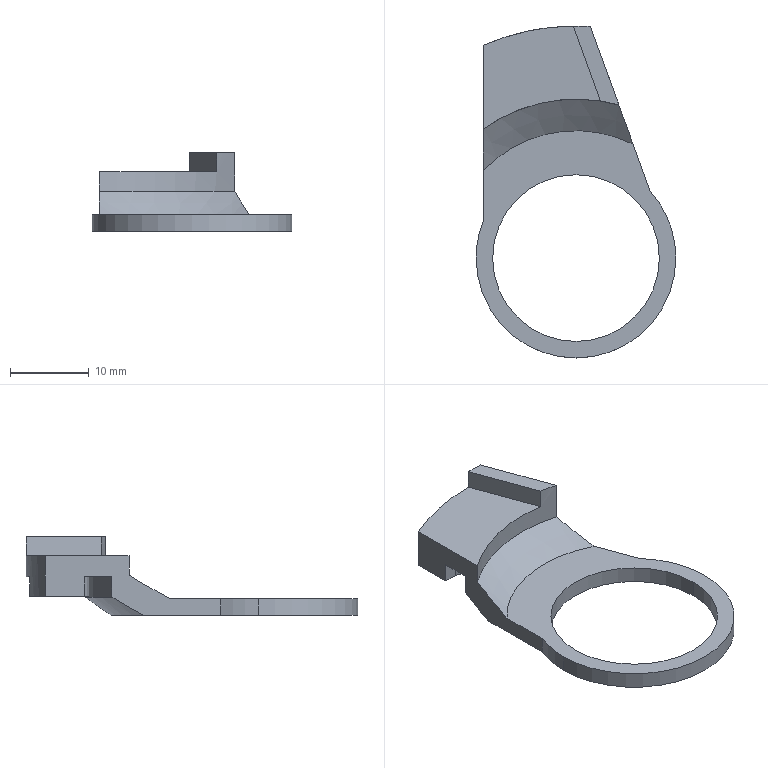Part | STEP file | A22NZ_H_02_LEVER | 1 solid | 23 faces | box 25.4 x 42.2 x 10 mm | volume 1414 mm3 | plane 11 | cylinder 10 | cone 2 | commonest cylinder face diameters 25.4 x3 7.5 x2 21.2 x2 40.4 x1 44 x1 59 x1
STEP:
#1=CARTESIAN_POINT('',(-4.25,25.26,0.3));
#2=VERTEX_POINT('',#1);
#3=CARTESIAN_POINT('',(-10.035,22.11,0.3));
#4=VERTEX_POINT('',#3);
#5=CARTESIAN_POINT('',(-8.,25.26,0.3));
#6=DIRECTION('',(0.,0.,-1.));
#7=DIRECTION('',(-1.,0.,0.));
#8=AXIS2_PLACEMENT_3D('',#5,#6,#7);
#9=CIRCLE('',#8,3.75);
#10=EDGE_CURVE('',#2,#4,#9,.T.);
#11=ORIENTED_EDGE('',*,*,#10,.F.);
#12=CARTESIAN_POINT('',(-4.25,25.26,2.8));
#13=VERTEX_POINT('',#12);
#14=CARTESIAN_POINT('',(-4.25,25.26,0.3));
#15=DIRECTION('',(0.,0.,1.));
#16=VECTOR('',#15,1000.);
#17=LINE('',#14,#16);
#18=EDGE_CURVE('',#2,#13,#17,.T.);
#19=ORIENTED_EDGE('',*,*,#18,.T.);
#20=CARTESIAN_POINT('',(-10.035,22.11,2.8));
#21=VERTEX_POINT('',#20);
#22=CARTESIAN_POINT('',(-8.,25.26,2.8));
#23=DIRECTION('',(0.,0.,-1.));
#24=DIRECTION('',(-1.,0.,0.));
#25=AXIS2_PLACEMENT_3D('',#22,#23,#24);
#26=CIRCLE('',#25,3.75);
#27=EDGE_CURVE('',#13,#21,#26,.T.);
#28=ORIENTED_EDGE('',*,*,#27,.T.);
#29=CARTESIAN_POINT('',(-10.035,22.11,0.3));
#30=DIRECTION('',(0.,0.,1.));
#31=VECTOR('',#30,1000.);
#32=LINE('',#29,#31);
#33=EDGE_CURVE('',#4,#21,#32,.T.);
#34=ORIENTED_EDGE('',*,*,#33,.F.);
#35=EDGE_LOOP('',(#11,#19,#28,#34));
#36=FACE_OUTER_BOUND('',#35,.T.);
#37=CARTESIAN_POINT('',(-8.,25.26,0.3));
#38=DIRECTION('',(0.,0.,1.));
#39=DIRECTION('',(1.,0.,0.));
#40=AXIS2_PLACEMENT_3D('',#37,#38,#39);
#41=CYLINDRICAL_SURFACE('',#40,3.75);
#42=ADVANCED_FACE('',(#36),#41,.T.);
#43=CARTESIAN_POINT('',(10.6,0.,-2.1));
#44=VERTEX_POINT('',#43);
#45=CARTESIAN_POINT('',(-10.6,0.,-2.1));
#46=VERTEX_POINT('',#45);
#47=CARTESIAN_POINT('',(0.,0.,-2.1));
#48=DIRECTION('',(0.,0.,-1.));
#49=DIRECTION('',(-1.,0.,0.));
#50=AXIS2_PLACEMENT_3D('',#47,#48,#49);
#51=CIRCLE('',#50,10.6);
#52=EDGE_CURVE('',#44,#46,#51,.T.);
#53=ORIENTED_EDGE('',*,*,#52,.T.);
#54=CARTESIAN_POINT('',(-10.6,0.,0.));
#55=VERTEX_POINT('',#54);
#56=CARTESIAN_POINT('',(-10.6,0.,-2.1));
#57=DIRECTION('',(0.,0.,1.));
#58=VECTOR('',#57,1000.);
#59=LINE('',#56,#58);
#60=EDGE_CURVE('',#46,#55,#59,.T.);
#61=ORIENTED_EDGE('',*,*,#60,.T.);
#62=CARTESIAN_POINT('',(10.6,0.,0.));
#63=VERTEX_POINT('',#62);
#64=CARTESIAN_POINT('',(0.,0.,0.));
#65=DIRECTION('',(0.,0.,-1.));
#66=DIRECTION('',(-1.,0.,0.));
#67=AXIS2_PLACEMENT_3D('',#64,#65,#66);
#68=CIRCLE('',#67,10.6);
#69=EDGE_CURVE('',#63,#55,#68,.T.);
#70=ORIENTED_EDGE('',*,*,#69,.F.);
#71=CARTESIAN_POINT('',(10.6,0.,-2.1));
#72=DIRECTION('',(0.,0.,1.));
#73=VECTOR('',#72,1000.);
#74=LINE('',#71,#73);
#75=EDGE_CURVE('',#44,#63,#74,.T.);
#76=ORIENTED_EDGE('',*,*,#75,.F.);
#77=EDGE_LOOP('',(#53,#61,#70,#76));
#78=FACE_OUTER_BOUND('',#77,.T.);
#79=CARTESIAN_POINT('',(0.,0.,-2.1));
#80=DIRECTION('',(0.,0.,1.));
#81=DIRECTION('',(1.,0.,0.));
#82=AXIS2_PLACEMENT_3D('',#79,#80,#81);
#83=CYLINDRICAL_SURFACE('',#82,10.6);
#84=ADVANCED_FACE('',(#78),#83,.F.);
#85=CARTESIAN_POINT('',(-12.7,0.,-2.1));
#86=VERTEX_POINT('',#85);
#87=CARTESIAN_POINT('',(-11.78,4.746,-2.1));
#88=VERTEX_POINT('',#87);
#89=CARTESIAN_POINT('',(0.,0.,-2.1));
#90=DIRECTION('',(0.,0.,-1.));
#91=DIRECTION('',(-1.,0.,0.));
#92=AXIS2_PLACEMENT_3D('',#89,#90,#91);
#93=CIRCLE('',#92,12.7);
#94=EDGE_CURVE('',#86,#88,#93,.T.);
#95=ORIENTED_EDGE('',*,*,#94,.F.);
#96=CARTESIAN_POINT('',(-12.7,0.,0.));
#97=VERTEX_POINT('',#96);
#98=CARTESIAN_POINT('',(-12.7,0.,-2.1));
#99=DIRECTION('',(0.,0.,1.));
#100=VECTOR('',#99,1000.);
#101=LINE('',#98,#100);
#102=EDGE_CURVE('',#86,#97,#101,.T.);
#103=ORIENTED_EDGE('',*,*,#102,.T.);
#104=CARTESIAN_POINT('',(-11.78,4.746,0.));
#105=VERTEX_POINT('',#104);
#106=CARTESIAN_POINT('',(0.,0.,0.));
#107=DIRECTION('',(0.,0.,-1.));
#108=DIRECTION('',(-1.,0.,0.));
#109=AXIS2_PLACEMENT_3D('',#106,#107,#108);
#110=CIRCLE('',#109,12.7);
#111=EDGE_CURVE('',#97,#105,#110,.T.);
#112=ORIENTED_EDGE('',*,*,#111,.T.);
#113=CARTESIAN_POINT('',(-11.78,4.746,-2.1));
#114=DIRECTION('',(0.,0.,1.));
#115=VECTOR('',#114,1000.);
#116=LINE('',#113,#115);
#117=EDGE_CURVE('',#88,#105,#116,.T.);
#118=ORIENTED_EDGE('',*,*,#117,.F.);
#119=EDGE_LOOP('',(#95,#103,#112,#118));
#120=FACE_OUTER_BOUND('',#119,.T.);
#121=CARTESIAN_POINT('',(0.,0.,-2.1));
#122=DIRECTION('',(0.,0.,1.));
#123=DIRECTION('',(1.,0.,0.));
#124=AXIS2_PLACEMENT_3D('',#121,#122,#123);
#125=CYLINDRICAL_SURFACE('',#124,12.7);
#126=ADVANCED_FACE('',(#120),#125,.T.);
#127=ORIENTED_EDGE('',*,*,#102,.F.);
#128=CARTESIAN_POINT('',(12.7,0.,-2.1));
#129=VERTEX_POINT('',#128);
#130=CARTESIAN_POINT('',(0.,0.,-2.1));
#131=DIRECTION('',(0.,0.,-1.));
#132=DIRECTION('',(-1.,0.,0.));
#133=AXIS2_PLACEMENT_3D('',#130,#131,#132);
#134=CIRCLE('',#133,12.7);
#135=EDGE_CURVE('',#129,#86,#134,.T.);
#136=ORIENTED_EDGE('',*,*,#135,.F.);
#137=CARTESIAN_POINT('',(12.7,0.,0.));
#138=VERTEX_POINT('',#137);
#139=CARTESIAN_POINT('',(12.7,0.,-2.1));
#140=DIRECTION('',(0.,0.,1.));
#141=VECTOR('',#140,1000.);
#142=LINE('',#139,#141);
#143=EDGE_CURVE('',#129,#138,#142,.T.);
#144=ORIENTED_EDGE('',*,*,#143,.T.);
#145=CARTESIAN_POINT('',(0.,0.,0.));
#146=DIRECTION('',(0.,0.,-1.));
#147=DIRECTION('',(-1.,0.,0.));
#148=AXIS2_PLACEMENT_3D('',#145,#146,#147);
#149=CIRCLE('',#148,12.7);
#150=EDGE_CURVE('',#138,#97,#149,.T.);
#151=ORIENTED_EDGE('',*,*,#150,.T.);
#152=EDGE_LOOP('',(#127,#136,#144,#151));
#153=FACE_OUTER_BOUND('',#152,.T.);
#154=CARTESIAN_POINT('',(0.,0.,-2.1));
#155=DIRECTION('',(0.,0.,1.));
#156=DIRECTION('',(1.,0.,0.));
#157=AXIS2_PLACEMENT_3D('',#154,#155,#156);
#158=CYLINDRICAL_SURFACE('',#157,12.7);
#159=ADVANCED_FACE('',(#153),#158,.T.);
#160=CARTESIAN_POINT('',(-11.78,22.11,2.8));
#161=VERTEX_POINT('',#160);
#162=CARTESIAN_POINT('',(-10.035,22.11,2.8));
#163=DIRECTION('',(-1.,0.,0.));
#164=VECTOR('',#163,1000.);
#165=LINE('',#162,#164);
#166=EDGE_CURVE('',#21,#161,#165,.T.);
#167=ORIENTED_EDGE('',*,*,#166,.F.);
#168=ORIENTED_EDGE('',*,*,#27,.F.);
#169=CARTESIAN_POINT('',(-5.25,27.81,2.8));
#170=VERTEX_POINT('',#169);
#171=CARTESIAN_POINT('',(-8.,25.26,2.8));
#172=DIRECTION('',(0.,0.,-1.));
#173=DIRECTION('',(-1.,0.,0.));
#174=AXIS2_PLACEMENT_3D('',#171,#172,#173);
#175=CIRCLE('',#174,3.75);
#176=EDGE_CURVE('',#170,#13,#175,.T.);
#177=ORIENTED_EDGE('',*,*,#176,.F.);
#178=CARTESIAN_POINT('',(-5.25,29.029,2.8));
#179=VERTEX_POINT('',#178);
#180=CARTESIAN_POINT('',(-5.25,27.81,2.8));
#181=DIRECTION('',(0.,-1.,0.));
#182=VECTOR('',#181,1000.);
#183=LINE('',#180,#182);
#184=EDGE_CURVE('',#179,#170,#183,.T.);
#185=ORIENTED_EDGE('',*,*,#184,.F.);
#186=CARTESIAN_POINT('',(1.816,29.444,2.8));
#187=VERTEX_POINT('',#186);
#188=CARTESIAN_POINT('',(0.,0.,2.8));
#189=DIRECTION('',(0.,0.,1.));
#190=DIRECTION('',(1.,0.,0.));
#191=AXIS2_PLACEMENT_3D('',#188,#189,#190);
#192=CIRCLE('',#191,29.5);
#193=EDGE_CURVE('',#187,#179,#192,.T.);
#194=ORIENTED_EDGE('',*,*,#193,.F.);
#195=CARTESIAN_POINT('',(4.711,21.49,2.8));
#196=VERTEX_POINT('',#195);
#197=CARTESIAN_POINT('',(5.454,19.45,2.8));
#198=DIRECTION('',(-0.342,0.9397,0.));
#199=VECTOR('',#198,1000.);
#200=LINE('',#197,#199);
#201=EDGE_CURVE('',#196,#187,#200,.T.);
#202=ORIENTED_EDGE('',*,*,#201,.F.);
#203=CARTESIAN_POINT('',(-11.78,18.58,2.8));
#204=VERTEX_POINT('',#203);
#205=CARTESIAN_POINT('',(0.,0.,2.8));
#206=DIRECTION('',(0.,0.,1.));
#207=DIRECTION('',(1.,0.,0.));
#208=AXIS2_PLACEMENT_3D('',#205,#206,#207);
#209=CIRCLE('',#208,22.);
#210=EDGE_CURVE('',#196,#204,#209,.T.);
#211=ORIENTED_EDGE('',*,*,#210,.T.);
#212=CARTESIAN_POINT('',(-11.78,18.58,2.8));
#213=DIRECTION('',(0.,1.,0.));
#214=VECTOR('',#213,1000.);
#215=LINE('',#212,#214);
#216=EDGE_CURVE('',#204,#161,#215,.T.);
#217=ORIENTED_EDGE('',*,*,#216,.T.);
#218=EDGE_LOOP('',(#167,#168,#177,#185,#194,#202,#211,#217));
#219=FACE_OUTER_BOUND('',#218,.T.);
#220=CARTESIAN_POINT('',(0.,0.,2.8));
#221=DIRECTION('',(0.,0.,1.));
#222=DIRECTION('',(1.,0.,0.));
#223=AXIS2_PLACEMENT_3D('',#220,#221,#222);
#224=PLANE('',#223);
#225=ADVANCED_FACE('',(#219),#224,.F.);
#226=CARTESIAN_POINT('',(4.711,21.49,0.2107));
#227=VERTEX_POINT('',#226);
#228=CARTESIAN_POINT('',(4.711,21.49,-2.1));
#229=DIRECTION('',(0.,0.,1.));
#230=VECTOR('',#229,1000.);
#231=LINE('',#228,#230);
#232=EDGE_CURVE('',#227,#196,#231,.T.);
#233=ORIENTED_EDGE('',*,*,#232,.F.);
#234=CARTESIAN_POINT('',(-11.78,18.58,0.2107));
#235=VERTEX_POINT('',#234);
#236=CARTESIAN_POINT('',(0.,0.,0.2107));
#237=DIRECTION('',(0.,0.,1.));
#238=DIRECTION('',(-1.,0.,0.));
#239=AXIS2_PLACEMENT_3D('',#236,#237,#238);
#240=CIRCLE('',#239,22.);
#241=EDGE_CURVE('',#227,#235,#240,.T.);
#242=ORIENTED_EDGE('',*,*,#241,.T.);
#243=CARTESIAN_POINT('',(-11.78,18.58,-2.1));
#244=DIRECTION('',(0.,0.,1.));
#245=VECTOR('',#244,1000.);
#246=LINE('',#243,#245);
#247=EDGE_CURVE('',#235,#204,#246,.T.);
#248=ORIENTED_EDGE('',*,*,#247,.T.);
#249=ORIENTED_EDGE('',*,*,#210,.F.);
#250=EDGE_LOOP('',(#233,#242,#248,#249));
#251=FACE_OUTER_BOUND('',#250,.T.);
#252=CARTESIAN_POINT('',(0.,0.,-2.1));
#253=DIRECTION('',(0.,0.,1.));
#254=DIRECTION('',(1.,0.,0.));
#255=AXIS2_PLACEMENT_3D('',#252,#253,#254);
#256=CYLINDRICAL_SURFACE('',#255,22.);
#257=ADVANCED_FACE('',(#251),#256,.T.);
#258=CARTESIAN_POINT('',(-11.78,16.409,5.5));
#259=VERTEX_POINT('',#258);
#260=CARTESIAN_POINT('',(3.142,19.954,5.5));
#261=VERTEX_POINT('',#260);
#262=CARTESIAN_POINT('',(0.,0.,5.5));
#263=DIRECTION('',(0.,0.,-1.));
#264=DIRECTION('',(1.,0.,0.));
#265=AXIS2_PLACEMENT_3D('',#262,#263,#264);
#266=CIRCLE('',#265,20.2);
#267=EDGE_CURVE('',#259,#261,#266,.T.);
#268=ORIENTED_EDGE('',*,*,#267,.T.);
#269=CARTESIAN_POINT('',(-0.332,29.498,5.5));
#270=VERTEX_POINT('',#269);
#271=CARTESIAN_POINT('',(9.187,3.344,5.5));
#272=DIRECTION('',(-0.342,0.9397,0.));
#273=VECTOR('',#272,1000.);
#274=LINE('',#271,#273);
#275=EDGE_CURVE('',#261,#270,#274,.T.);
#276=ORIENTED_EDGE('',*,*,#275,.T.);
#277=CARTESIAN_POINT('',(-11.78,27.046,5.5));
#278=VERTEX_POINT('',#277);
#279=CARTESIAN_POINT('',(0.,0.,5.5));
#280=DIRECTION('',(0.,0.,-1.));
#281=DIRECTION('',(1.,0.,0.));
#282=AXIS2_PLACEMENT_3D('',#279,#280,#281);
#283=CIRCLE('',#282,29.5);
#284=EDGE_CURVE('',#278,#270,#283,.T.);
#285=ORIENTED_EDGE('',*,*,#284,.F.);
#286=CARTESIAN_POINT('',(-11.78,16.409,5.5));
#287=DIRECTION('',(0.,-1.,0.));
#288=VECTOR('',#287,1000.);
#289=LINE('',#286,#288);
#290=EDGE_CURVE('',#278,#259,#289,.T.);
#291=ORIENTED_EDGE('',*,*,#290,.T.);
#292=EDGE_LOOP('',(#268,#276,#285,#291));
#293=FACE_OUTER_BOUND('',#292,.T.);
#294=CARTESIAN_POINT('',(0.,0.,5.5));
#295=DIRECTION('',(0.,0.,1.));
#296=DIRECTION('',(1.,0.,0.));
#297=AXIS2_PLACEMENT_3D('',#294,#295,#296);
#298=PLANE('',#297);
#299=ADVANCED_FACE('',(#293),#298,.T.);
#300=ORIENTED_EDGE('',*,*,#69,.T.);
#301=CARTESIAN_POINT('',(0.,0.,0.));
#302=DIRECTION('',(0.,0.,-1.));
#303=DIRECTION('',(-1.,0.,0.));
#304=AXIS2_PLACEMENT_3D('',#301,#302,#303);
#305=CIRCLE('',#304,10.6);
#306=EDGE_CURVE('',#55,#63,#305,.T.);
#307=ORIENTED_EDGE('',*,*,#306,.T.);
#308=EDGE_LOOP('',(#300,#307));
#309=FACE_BOUND('',#308,.T.);
#310=CARTESIAN_POINT('',(7.262,14.481,0.));
#311=VERTEX_POINT('',#310);
#312=CARTESIAN_POINT('',(9.441,8.495,0.));
#313=VERTEX_POINT('',#312);
#314=CARTESIAN_POINT('',(9.441,8.495,0.));
#315=DIRECTION('',(0.342,-0.9397,0.));
#316=VECTOR('',#315,1000.);
#317=LINE('',#314,#316);
#318=EDGE_CURVE('',#311,#313,#317,.T.);
#319=ORIENTED_EDGE('',*,*,#318,.F.);
#320=CARTESIAN_POINT('',(-11.78,11.121,0.));
#321=VERTEX_POINT('',#320);
#322=CARTESIAN_POINT('',(0.,0.,0.));
#323=DIRECTION('',(0.,0.,1.));
#324=DIRECTION('',(-1.,0.,0.));
#325=AXIS2_PLACEMENT_3D('',#322,#323,#324);
#326=CIRCLE('',#325,16.2);
#327=EDGE_CURVE('',#311,#321,#326,.T.);
#328=ORIENTED_EDGE('',*,*,#327,.T.);
#329=CARTESIAN_POINT('',(-11.78,4.746,0.));
#330=DIRECTION('',(0.,1.,0.));
#331=VECTOR('',#330,1000.);
#332=LINE('',#329,#331);
#333=EDGE_CURVE('',#105,#321,#332,.T.);
#334=ORIENTED_EDGE('',*,*,#333,.F.);
#335=ORIENTED_EDGE('',*,*,#111,.F.);
#336=ORIENTED_EDGE('',*,*,#150,.F.);
#337=CARTESIAN_POINT('',(0.,0.,0.));
#338=DIRECTION('',(0.,0.,-1.));
#339=DIRECTION('',(-1.,0.,0.));
#340=AXIS2_PLACEMENT_3D('',#337,#338,#339);
#341=CIRCLE('',#340,12.7);
#342=EDGE_CURVE('',#313,#138,#341,.T.);
#343=ORIENTED_EDGE('',*,*,#342,.F.);
#344=EDGE_LOOP('',(#319,#328,#334,#335,#336,#343));
#345=FACE_OUTER_BOUND('',#344,.T.);
#346=CARTESIAN_POINT('',(0.,0.,0.));
#347=DIRECTION('',(0.,0.,-1.));
#348=DIRECTION('',(-1.,0.,0.));
#349=AXIS2_PLACEMENT_3D('',#346,#347,#348);
#350=PLANE('',#349);
#351=ADVANCED_FACE('',(#309,#345),#350,.F.);
#352=CARTESIAN_POINT('',(-11.78,14.523,-2.1));
#353=VERTEX_POINT('',#352);
#354=CARTESIAN_POINT('',(-11.78,4.746,-2.1));
#355=DIRECTION('',(0.,1.,0.));
#356=VECTOR('',#355,1000.);
#357=LINE('',#354,#356);
#358=EDGE_CURVE('',#88,#353,#357,.T.);
#359=ORIENTED_EDGE('',*,*,#358,.T.);
#360=CARTESIAN_POINT('',(6.099,17.678,-2.1));
#361=VERTEX_POINT('',#360);
#362=CARTESIAN_POINT('',(0.,0.,-2.1));
#363=DIRECTION('',(0.,0.,-1.));
#364=DIRECTION('',(-1.,0.,0.));
#365=AXIS2_PLACEMENT_3D('',#362,#363,#364);
#366=CIRCLE('',#365,18.7);
#367=EDGE_CURVE('',#353,#361,#366,.T.);
#368=ORIENTED_EDGE('',*,*,#367,.T.);
#369=CARTESIAN_POINT('',(9.441,8.495,-2.1));
#370=VERTEX_POINT('',#369);
#371=CARTESIAN_POINT('',(9.441,8.495,-2.1));
#372=DIRECTION('',(0.342,-0.9397,0.));
#373=VECTOR('',#372,1000.);
#374=LINE('',#371,#373);
#375=EDGE_CURVE('',#361,#370,#374,.T.);
#376=ORIENTED_EDGE('',*,*,#375,.T.);
#377=CARTESIAN_POINT('',(0.,0.,-2.1));
#378=DIRECTION('',(0.,0.,-1.));
#379=DIRECTION('',(-1.,0.,0.));
#380=AXIS2_PLACEMENT_3D('',#377,#378,#379);
#381=CIRCLE('',#380,12.7);
#382=EDGE_CURVE('',#370,#129,#381,.T.);
#383=ORIENTED_EDGE('',*,*,#382,.T.);
#384=ORIENTED_EDGE('',*,*,#135,.T.);
#385=ORIENTED_EDGE('',*,*,#94,.T.);
#386=EDGE_LOOP('',(#359,#368,#376,#383,#384,#385));
#387=FACE_OUTER_BOUND('',#386,.T.);
#388=ORIENTED_EDGE('',*,*,#52,.F.);
#389=CARTESIAN_POINT('',(0.,0.,-2.1));
#390=DIRECTION('',(0.,0.,-1.));
#391=DIRECTION('',(-1.,0.,0.));
#392=AXIS2_PLACEMENT_3D('',#389,#390,#391);
#393=CIRCLE('',#392,10.6);
#394=EDGE_CURVE('',#46,#44,#393,.T.);
#395=ORIENTED_EDGE('',*,*,#394,.F.);
#396=EDGE_LOOP('',(#388,#395));
#397=FACE_BOUND('',#396,.T.);
#398=CARTESIAN_POINT('',(0.,0.,-2.1));
#399=DIRECTION('',(0.,0.,-1.));
#400=DIRECTION('',(-1.,0.,0.));
#401=AXIS2_PLACEMENT_3D('',#398,#399,#400);
#402=PLANE('',#401);
#403=ADVANCED_FACE('',(#387,#397),#402,.T.);
#404=ORIENTED_EDGE('',*,*,#143,.F.);
#405=ORIENTED_EDGE('',*,*,#382,.F.);
#406=CARTESIAN_POINT('',(9.441,8.495,-2.1));
#407=DIRECTION('',(0.,0.,1.));
#408=VECTOR('',#407,1000.);
#409=LINE('',#406,#408);
#410=EDGE_CURVE('',#370,#313,#409,.T.);
#411=ORIENTED_EDGE('',*,*,#410,.T.);
#412=ORIENTED_EDGE('',*,*,#342,.T.);
#413=EDGE_LOOP('',(#404,#405,#411,#412));
#414=FACE_OUTER_BOUND('',#413,.T.);
#415=CARTESIAN_POINT('',(0.,0.,-2.1));
#416=DIRECTION('',(0.,0.,1.));
#417=DIRECTION('',(1.,0.,0.));
#418=AXIS2_PLACEMENT_3D('',#415,#416,#417);
#419=CYLINDRICAL_SURFACE('',#418,12.7);
#420=ADVANCED_FACE('',(#414),#419,.T.);
#421=ORIENTED_EDGE('',*,*,#247,.F.);
#422=CARTESIAN_POINT('',(-11.78,18.58,0.2107));
#423=CARTESIAN_POINT('',(-11.78,17.241,-0.5817));
#424=CARTESIAN_POINT('',(-11.78,15.891,-1.356));
#425=CARTESIAN_POINT('',(-11.78,14.523,-2.1));
#426=B_SPLINE_CURVE_WITH_KNOTS('',3,(#422,#423,#424,#425),.UNSPECIFIED.,.F.,.F.,(4,4),(0.,0.004669),.UNSPECIFIED.);
#427=EDGE_CURVE('',#235,#353,#426,.T.);
#428=ORIENTED_EDGE('',*,*,#427,.T.);
#429=ORIENTED_EDGE('',*,*,#358,.F.);
#430=ORIENTED_EDGE('',*,*,#117,.T.);
#431=ORIENTED_EDGE('',*,*,#333,.T.);
#432=CARTESIAN_POINT('',(-11.78,16.409,3.));
#433=VERTEX_POINT('',#432);
#434=CARTESIAN_POINT('',(-11.78,11.121,0.));
#435=CARTESIAN_POINT('',(-11.78,12.924,0.9285));
#436=CARTESIAN_POINT('',(-11.78,14.678,1.945));
#437=CARTESIAN_POINT('',(-11.78,16.409,3.));
#438=B_SPLINE_CURVE_WITH_KNOTS('',3,(#434,#435,#436,#437),.UNSPECIFIED.,.F.,.F.,(4,4),(0.,0.00608),.UNSPECIFIED.);
#439=EDGE_CURVE('',#321,#433,#438,.T.);
#440=ORIENTED_EDGE('',*,*,#439,.T.);
#441=CARTESIAN_POINT('',(-11.78,16.409,5.5));
#442=DIRECTION('',(0.,0.,-1.));
#443=VECTOR('',#442,1000.);
#444=LINE('',#441,#443);
#445=EDGE_CURVE('',#259,#433,#444,.T.);
#446=ORIENTED_EDGE('',*,*,#445,.F.);
#447=ORIENTED_EDGE('',*,*,#290,.F.);
#448=CARTESIAN_POINT('',(-11.78,27.046,0.3));
#449=VERTEX_POINT('',#448);
#450=CARTESIAN_POINT('',(-11.78,27.046,23.433));
#451=DIRECTION('',(0.,0.,-1.));
#452=VECTOR('',#451,1000.);
#453=LINE('',#450,#452);
#454=EDGE_CURVE('',#278,#449,#453,.T.);
#455=ORIENTED_EDGE('',*,*,#454,.T.);
#456=CARTESIAN_POINT('',(-11.78,22.11,0.3));
#457=VERTEX_POINT('',#456);
#458=CARTESIAN_POINT('',(-11.78,22.11,0.3));
#459=DIRECTION('',(0.,1.,0.));
#460=VECTOR('',#459,1000.);
#461=LINE('',#458,#460);
#462=EDGE_CURVE('',#457,#449,#461,.T.);
#463=ORIENTED_EDGE('',*,*,#462,.F.);
#464=CARTESIAN_POINT('',(-11.78,22.11,0.3));
#465=DIRECTION('',(0.,0.,1.));
#466=VECTOR('',#465,1000.);
#467=LINE('',#464,#466);
#468=EDGE_CURVE('',#457,#161,#467,.T.);
#469=ORIENTED_EDGE('',*,*,#468,.T.);
#470=ORIENTED_EDGE('',*,*,#216,.F.);
#471=EDGE_LOOP('',(#421,#428,#429,#430,#431,#440,#446,#447,#455,#463,#469,#470));
#472=FACE_OUTER_BOUND('',#471,.T.);
#473=CARTESIAN_POINT('',(-11.78,4.746,-2.1));
#474=DIRECTION('',(1.,0.,0.));
#475=DIRECTION('',(0.,0.,-1.));
#476=AXIS2_PLACEMENT_3D('',#473,#474,#475);
#477=PLANE('',#476);
#478=ADVANCED_FACE('',(#472),#477,.F.);
#479=ORIENTED_EDGE('',*,*,#375,.F.);
#480=CARTESIAN_POINT('',(6.099,17.678,-2.1));
#481=CARTESIAN_POINT('',(5.631,18.962,-1.356));
#482=CARTESIAN_POINT('',(5.169,20.231,-0.5816));
#483=CARTESIAN_POINT('',(4.711,21.49,0.2107));
#484=B_SPLINE_CURVE_WITH_KNOTS('',3,(#480,#481,#482,#483),.UNSPECIFIED.,.F.,.F.,(4,4),(0.,0.004669),.UNSPECIFIED.);
#485=EDGE_CURVE('',#361,#227,#484,.T.);
#486=ORIENTED_EDGE('',*,*,#485,.T.);
#487=ORIENTED_EDGE('',*,*,#232,.T.);
#488=ORIENTED_EDGE('',*,*,#201,.T.);
#489=CARTESIAN_POINT('',(1.816,29.444,7.9));
#490=VERTEX_POINT('',#489);
#491=CARTESIAN_POINT('',(1.816,29.444,7.9));
#492=DIRECTION('',(0.,0.,-1.));
#493=VECTOR('',#492,1000.);
#494=LINE('',#491,#493);
#495=EDGE_CURVE('',#490,#187,#494,.T.);
#496=ORIENTED_EDGE('',*,*,#495,.F.);
#497=CARTESIAN_POINT('',(5.454,19.45,7.9));
#498=VERTEX_POINT('',#497);
#499=CARTESIAN_POINT('',(5.454,19.45,7.9));
#500=DIRECTION('',(-0.342,0.9397,0.));
#501=VECTOR('',#500,1000.);
#502=LINE('',#499,#501);
#503=EDGE_CURVE('',#498,#490,#502,.T.);
#504=ORIENTED_EDGE('',*,*,#503,.F.);
#505=CARTESIAN_POINT('',(5.454,19.45,3.));
#506=VERTEX_POINT('',#505);
#507=CARTESIAN_POINT('',(5.454,19.45,5.5));
#508=DIRECTION('',(0.,0.,-1.));
#509=VECTOR('',#508,1000.);
#510=LINE('',#507,#509);
#511=EDGE_CURVE('',#498,#506,#510,.T.);
#512=ORIENTED_EDGE('',*,*,#511,.T.);
#513=CARTESIAN_POINT('',(5.454,19.45,3.));
#514=CARTESIAN_POINT('',(6.046,17.823,1.945));
#515=CARTESIAN_POINT('',(6.645,16.175,0.9286));
#516=CARTESIAN_POINT('',(7.262,14.481,0.));
#517=B_SPLINE_CURVE_WITH_KNOTS('',3,(#513,#514,#515,#516),.UNSPECIFIED.,.F.,.F.,(4,4),(0.,0.006079),.UNSPECIFIED.);
#518=EDGE_CURVE('',#506,#311,#517,.T.);
#519=ORIENTED_EDGE('',*,*,#518,.T.);
#520=ORIENTED_EDGE('',*,*,#318,.T.);
#521=ORIENTED_EDGE('',*,*,#410,.F.);
#522=EDGE_LOOP('',(#479,#486,#487,#488,#496,#504,#512,#519,#520,#521));
#523=FACE_OUTER_BOUND('',#522,.T.);
#524=CARTESIAN_POINT('',(9.441,8.495,-2.1));
#525=DIRECTION('',(-0.9397,-0.342,0.));
#526=DIRECTION('',(0.342,-0.9397,0.));
#527=AXIS2_PLACEMENT_3D('',#524,#525,#526);
#528=PLANE('',#527);
#529=ADVANCED_FACE('',(#523),#528,.F.);
#530=ORIENTED_EDGE('',*,*,#60,.F.);
#531=ORIENTED_EDGE('',*,*,#394,.T.);
#532=ORIENTED_EDGE('',*,*,#75,.T.);
#533=ORIENTED_EDGE('',*,*,#306,.F.);
#534=EDGE_LOOP('',(#530,#531,#532,#533));
#535=FACE_OUTER_BOUND('',#534,.T.);
#536=CARTESIAN_POINT('',(0.,0.,-2.1));
#537=DIRECTION('',(0.,0.,1.));
#538=DIRECTION('',(1.,0.,0.));
#539=AXIS2_PLACEMENT_3D('',#536,#537,#538);
#540=CYLINDRICAL_SURFACE('',#539,10.6);
#541=ADVANCED_FACE('',(#535),#540,.F.);
#542=ORIENTED_EDGE('',*,*,#445,.T.);
#543=CARTESIAN_POINT('',(0.,0.,3.));
#544=DIRECTION('',(0.,0.,-1.));
#545=DIRECTION('',(-1.,0.,0.));
#546=AXIS2_PLACEMENT_3D('',#543,#544,#545);
#547=CIRCLE('',#546,20.2);
#548=EDGE_CURVE('',#433,#506,#547,.T.);
#549=ORIENTED_EDGE('',*,*,#548,.T.);
#550=ORIENTED_EDGE('',*,*,#511,.F.);
#551=CARTESIAN_POINT('',(3.142,19.954,7.9));
#552=VERTEX_POINT('',#551);
#553=CARTESIAN_POINT('',(0.,0.,7.9));
#554=DIRECTION('',(0.,0.,-1.));
#555=DIRECTION('',(1.,0.,0.));
#556=AXIS2_PLACEMENT_3D('',#553,#554,#555);
#557=CIRCLE('',#556,20.2);
#558=EDGE_CURVE('',#552,#498,#557,.T.);
#559=ORIENTED_EDGE('',*,*,#558,.F.);
#560=CARTESIAN_POINT('',(3.142,19.954,7.9));
#561=DIRECTION('',(0.,0.,-1.));
#562=VECTOR('',#561,1000.);
#563=LINE('',#560,#562);
#564=EDGE_CURVE('',#552,#261,#563,.T.);
#565=ORIENTED_EDGE('',*,*,#564,.T.);
#566=ORIENTED_EDGE('',*,*,#267,.F.);
#567=EDGE_LOOP('',(#542,#549,#550,#559,#565,#566));
#568=FACE_OUTER_BOUND('',#567,.T.);
#569=CARTESIAN_POINT('',(0.,0.,5.5));
#570=DIRECTION('',(0.,0.,-1.));
#571=DIRECTION('',(-1.,0.,0.));
#572=AXIS2_PLACEMENT_3D('',#569,#570,#571);
#573=CYLINDRICAL_SURFACE('',#572,20.2);
#574=ADVANCED_FACE('',(#568),#573,.F.);
#575=CARTESIAN_POINT('',(-0.332,29.498,7.9));
#576=VERTEX_POINT('',#575);
#577=CARTESIAN_POINT('',(-0.332,29.498,7.9));
#578=DIRECTION('',(0.,0.,-1.));
#579=VECTOR('',#578,1000.);
#580=LINE('',#577,#579);
#581=EDGE_CURVE('',#576,#270,#580,.T.);
#582=ORIENTED_EDGE('',*,*,#581,.T.);
#583=ORIENTED_EDGE('',*,*,#275,.F.);
#584=ORIENTED_EDGE('',*,*,#564,.F.);
#585=CARTESIAN_POINT('',(3.142,19.954,7.9));
#586=DIRECTION('',(0.342,-0.9397,0.));
#587=VECTOR('',#586,1000.);
#588=LINE('',#585,#587);
#589=EDGE_CURVE('',#576,#552,#588,.T.);
#590=ORIENTED_EDGE('',*,*,#589,.F.);
#591=EDGE_LOOP('',(#582,#583,#584,#590));
#592=FACE_OUTER_BOUND('',#591,.T.);
#593=CARTESIAN_POINT('',(3.142,19.954,7.9));
#594=DIRECTION('',(0.9397,0.342,0.));
#595=DIRECTION('',(-0.342,0.9397,0.));
#596=AXIS2_PLACEMENT_3D('',#593,#594,#595);
#597=PLANE('',#596);
#598=ADVANCED_FACE('',(#592),#597,.F.);
#599=ORIENTED_EDGE('',*,*,#495,.T.);
#600=ORIENTED_EDGE('',*,*,#193,.T.);
#601=CARTESIAN_POINT('',(-5.25,29.029,0.3));
#602=VERTEX_POINT('',#601);
#603=CARTESIAN_POINT('',(-5.25,29.029,0.3));
#604=DIRECTION('',(0.,0.,1.));
#605=VECTOR('',#604,1000.);
#606=LINE('',#603,#605);
#607=EDGE_CURVE('',#602,#179,#606,.T.);
#608=ORIENTED_EDGE('',*,*,#607,.F.);
#609=CARTESIAN_POINT('',(0.,0.,0.3));
#610=DIRECTION('',(0.,0.,-1.));
#611=DIRECTION('',(-1.,0.,0.));
#612=AXIS2_PLACEMENT_3D('',#609,#610,#611);
#613=CIRCLE('',#612,29.5);
#614=EDGE_CURVE('',#449,#602,#613,.T.);
#615=ORIENTED_EDGE('',*,*,#614,.F.);
#616=ORIENTED_EDGE('',*,*,#454,.F.);
#617=ORIENTED_EDGE('',*,*,#284,.T.);
#618=ORIENTED_EDGE('',*,*,#581,.F.);
#619=CARTESIAN_POINT('',(0.,0.,7.9));
#620=DIRECTION('',(0.,0.,1.));
#621=DIRECTION('',(1.,0.,0.));
#622=AXIS2_PLACEMENT_3D('',#619,#620,#621);
#623=CIRCLE('',#622,29.5);
#624=EDGE_CURVE('',#490,#576,#623,.T.);
#625=ORIENTED_EDGE('',*,*,#624,.F.);
#626=EDGE_LOOP('',(#599,#600,#608,#615,#616,#617,#618,#625));
#627=FACE_OUTER_BOUND('',#626,.T.);
#628=CARTESIAN_POINT('',(0.,0.,7.9));
#629=DIRECTION('',(0.,0.,-1.));
#630=DIRECTION('',(-1.,0.,0.));
#631=AXIS2_PLACEMENT_3D('',#628,#629,#630);
#632=CYLINDRICAL_SURFACE('',#631,29.5);
#633=ADVANCED_FACE('',(#627),#632,.T.);
#634=ORIENTED_EDGE('',*,*,#558,.T.);
#635=ORIENTED_EDGE('',*,*,#503,.T.);
#636=ORIENTED_EDGE('',*,*,#624,.T.);
#637=ORIENTED_EDGE('',*,*,#589,.T.);
#638=EDGE_LOOP('',(#634,#635,#636,#637));
#639=FACE_OUTER_BOUND('',#638,.T.);
#640=CARTESIAN_POINT('',(0.,0.,7.9));
#641=DIRECTION('',(0.,0.,1.));
#642=DIRECTION('',(1.,0.,0.));
#643=AXIS2_PLACEMENT_3D('',#640,#641,#642);
#644=PLANE('',#643);
#645=ADVANCED_FACE('',(#639),#644,.T.);
#646=ORIENTED_EDGE('',*,*,#18,.F.);
#647=CARTESIAN_POINT('',(-5.25,27.81,0.3));
#648=VERTEX_POINT('',#647);
#649=CARTESIAN_POINT('',(-8.,25.26,0.3));
#650=DIRECTION('',(0.,0.,-1.));
#651=DIRECTION('',(-1.,0.,0.));
#652=AXIS2_PLACEMENT_3D('',#649,#650,#651);
#653=CIRCLE('',#652,3.75);
#654=EDGE_CURVE('',#648,#2,#653,.T.);
#655=ORIENTED_EDGE('',*,*,#654,.F.);
#656=CARTESIAN_POINT('',(-5.25,27.81,0.3));
#657=DIRECTION('',(0.,0.,1.));
#658=VECTOR('',#657,1000.);
#659=LINE('',#656,#658);
#660=EDGE_CURVE('',#648,#170,#659,.T.);
#661=ORIENTED_EDGE('',*,*,#660,.T.);
#662=ORIENTED_EDGE('',*,*,#176,.T.);
#663=EDGE_LOOP('',(#646,#655,#661,#662));
#664=FACE_OUTER_BOUND('',#663,.T.);
#665=CARTESIAN_POINT('',(-8.,25.26,0.3));
#666=DIRECTION('',(0.,0.,1.));
#667=DIRECTION('',(1.,0.,0.));
#668=AXIS2_PLACEMENT_3D('',#665,#666,#667);
#669=CYLINDRICAL_SURFACE('',#668,3.75);
#670=ADVANCED_FACE('',(#664),#669,.T.);
#671=ORIENTED_EDGE('',*,*,#166,.T.);
#672=ORIENTED_EDGE('',*,*,#468,.F.);
#673=CARTESIAN_POINT('',(-10.035,22.11,0.3));
#674=DIRECTION('',(-1.,0.,0.));
#675=VECTOR('',#674,1000.);
#676=LINE('',#673,#675);
#677=EDGE_CURVE('',#4,#457,#676,.T.);
#678=ORIENTED_EDGE('',*,*,#677,.F.);
#679=ORIENTED_EDGE('',*,*,#33,.T.);
#680=EDGE_LOOP('',(#671,#672,#678,#679));
#681=FACE_OUTER_BOUND('',#680,.T.);
#682=CARTESIAN_POINT('',(-10.035,22.11,0.3));
#683=DIRECTION('',(0.,1.,0.));
#684=DIRECTION('',(0.,0.,1.));
#685=AXIS2_PLACEMENT_3D('',#682,#683,#684);
#686=PLANE('',#685);
#687=ADVANCED_FACE('',(#681),#686,.F.);
#688=ORIENTED_EDGE('',*,*,#184,.T.);
#689=ORIENTED_EDGE('',*,*,#660,.F.);
#690=CARTESIAN_POINT('',(-5.25,27.81,0.3));
#691=DIRECTION('',(0.,-1.,0.));
#692=VECTOR('',#691,1000.);
#693=LINE('',#690,#692);
#694=EDGE_CURVE('',#602,#648,#693,.T.);
#695=ORIENTED_EDGE('',*,*,#694,.F.);
#696=ORIENTED_EDGE('',*,*,#607,.T.);
#697=EDGE_LOOP('',(#688,#689,#695,#696));
#698=FACE_OUTER_BOUND('',#697,.T.);
#699=CARTESIAN_POINT('',(-5.25,27.81,0.3));
#700=DIRECTION('',(-1.,0.,0.));
#701=DIRECTION('',(0.,0.,1.));
#702=AXIS2_PLACEMENT_3D('',#699,#700,#701);
#703=PLANE('',#702);
#704=ADVANCED_FACE('',(#698),#703,.F.);
#705=ORIENTED_EDGE('',*,*,#654,.T.);
#706=ORIENTED_EDGE('',*,*,#10,.T.);
#707=ORIENTED_EDGE('',*,*,#677,.T.);
#708=ORIENTED_EDGE('',*,*,#462,.T.);
#709=ORIENTED_EDGE('',*,*,#614,.T.);
#710=ORIENTED_EDGE('',*,*,#694,.T.);
#711=EDGE_LOOP('',(#705,#706,#707,#708,#709,#710));
#712=FACE_OUTER_BOUND('',#711,.T.);
#713=CARTESIAN_POINT('',(-8.,25.26,0.3));
#714=DIRECTION('',(0.,0.,-1.));
#715=DIRECTION('',(-1.,0.,0.));
#716=AXIS2_PLACEMENT_3D('',#713,#714,#715);
#717=PLANE('',#716);
#718=ADVANCED_FACE('',(#712),#717,.T.);
#719=ORIENTED_EDGE('',*,*,#427,.F.);
#720=ORIENTED_EDGE('',*,*,#241,.F.);
#721=ORIENTED_EDGE('',*,*,#485,.F.);
#722=ORIENTED_EDGE('',*,*,#367,.F.);
#723=EDGE_LOOP('',(#719,#720,#721,#722));
#724=FACE_OUTER_BOUND('',#723,.T.);
#725=CARTESIAN_POINT('',(0.,0.,-2.1));
#726=DIRECTION('',(0.,0.,1.));
#727=DIRECTION('',(1.,0.,0.));
#728=AXIS2_PLACEMENT_3D('',#725,#726,#727);
#729=CONICAL_SURFACE('',#728,18.7,0.9599);
#730=ADVANCED_FACE('',(#724),#729,.T.);
#731=ORIENTED_EDGE('',*,*,#439,.F.);
#732=ORIENTED_EDGE('',*,*,#327,.F.);
#733=ORIENTED_EDGE('',*,*,#518,.F.);
#734=ORIENTED_EDGE('',*,*,#548,.F.);
#735=EDGE_LOOP('',(#731,#732,#733,#734));
#736=FACE_OUTER_BOUND('',#735,.T.);
#737=CARTESIAN_POINT('',(0.,0.,3.));
#738=DIRECTION('',(0.,0.,1.));
#739=DIRECTION('',(1.,0.,0.));
#740=AXIS2_PLACEMENT_3D('',#737,#738,#739);
#741=CONICAL_SURFACE('',#740,20.2,0.9273);
#742=ADVANCED_FACE('',(#736),#741,.F.);
#743=CLOSED_SHELL('',(#42,#84,#126,#159,#225,#257,#299,#351,#403,#420,#478,#529,#541,#574,#598,#633,#645,#670,#687,#704,#718,#730,#742));
#744=MANIFOLD_SOLID_BREP('',#743);
#745=CARTESIAN_POINT('',(0.,0.,0.));
#746=DIRECTION('',(0.,0.,1.));
#747=DIRECTION('',(1.,0.,0.));
#748=AXIS2_PLACEMENT_3D('',#745,#746,#747);
#749=(LENGTH_UNIT()NAMED_UNIT(*)SI_UNIT(.MILLI.,.METRE.));
#750=UNCERTAINTY_MEASURE_WITH_UNIT(LENGTH_MEASURE(0.00001),#749,'','');
#751=(NAMED_UNIT(*)PLANE_ANGLE_UNIT()SI_UNIT($,.RADIAN.));
#752=(NAMED_UNIT(*)SI_UNIT($,.STERADIAN.)SOLID_ANGLE_UNIT());
#753=(GEOMETRIC_REPRESENTATION_CONTEXT(3)GLOBAL_UNCERTAINTY_ASSIGNED_CONTEXT((#750))GLOBAL_UNIT_ASSIGNED_CONTEXT((#749,#751,#752))REPRESENTATION_CONTEXT('',''));
#754=ADVANCED_BREP_SHAPE_REPRESENTATION('',(#744,#748),#753);